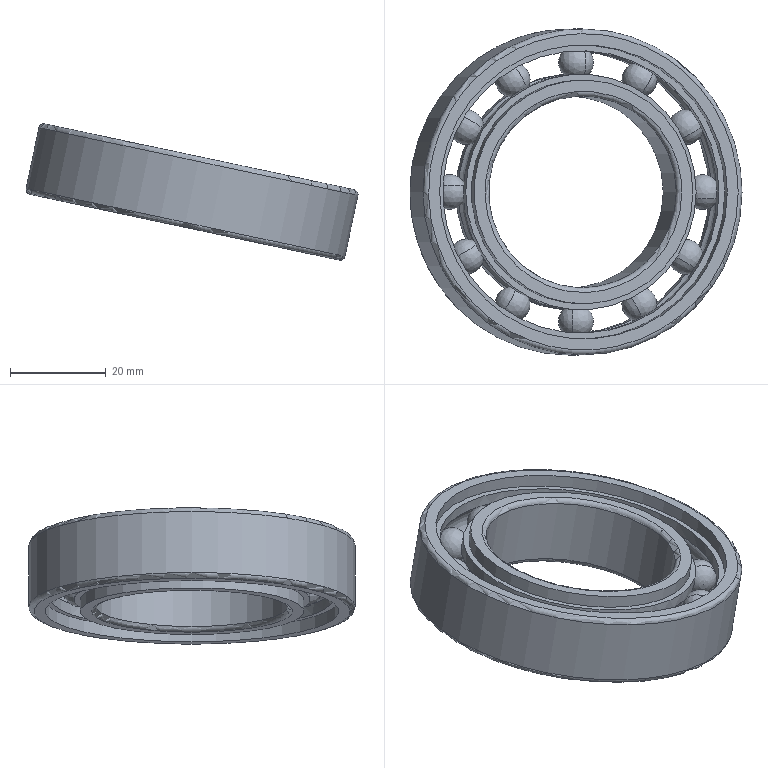Part | STEP file | 8903-ZC6008-2RS bearing 6008-2Z | 14 solids | 70 faces | box 69.261 x 68 x 28.438 mm | volume 22880 mm3 | torus 28 | sphere 24 | cylinder 10 | plane 8 | commonest cylinder face diameters 46.672 x2 49.128 x2 58.872 x2 61.328 x2 40 x1 68 x1